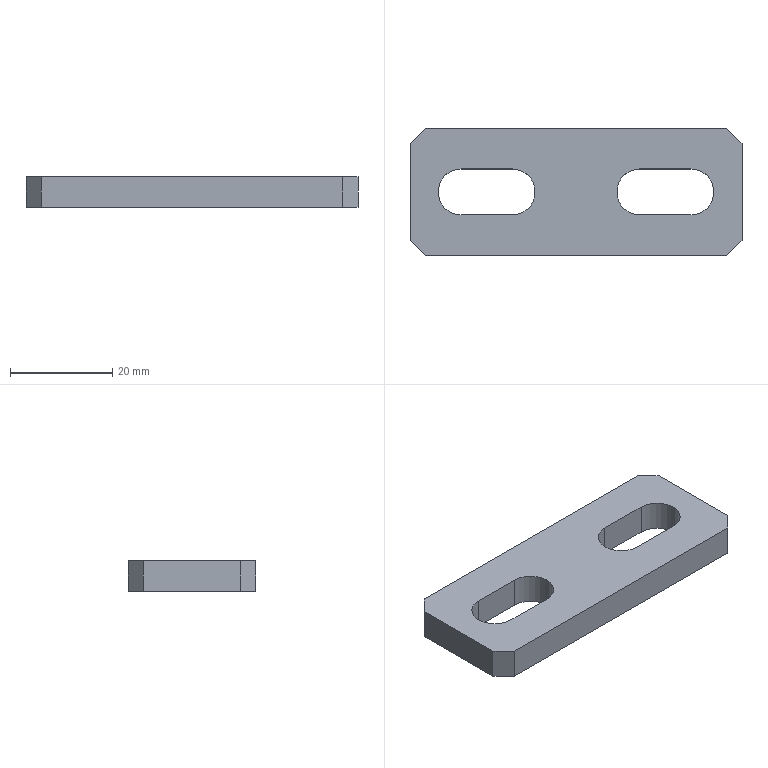Part | STEP file | linkfor guide | 1 solid | 18 faces | box 65 x 25 x 6 mm | volume 7799 mm3 | plane 14 | cylinder 4 | commonest cylinder face diameters 9 x4
STEP:
#1=CARTESIAN_POINT('',(0.,0.,0.));
#2=DIRECTION('',(0.,0.,1.));
#3=DIRECTION('',(1.,0.,0.));
#4=AXIS2_PLACEMENT_3D('',#1,#2,#3);
#5=CARTESIAN_POINT('',(45.,-10.346,6.));
#6=VERTEX_POINT('',#5);
#7=CARTESIAN_POINT('',(45.,-10.346,0.));
#8=VERTEX_POINT('',#7);
#9=CARTESIAN_POINT('',(45.,-10.346,6.));
#10=DIRECTION('',(0.,0.,-1.));
#11=VECTOR('',#10,1.);
#12=LINE('',#9,#11);
#13=CARTESIAN_POINT('',(45.,-5.846,6.));
#14=DIRECTION('',(0.,0.,-1.));
#15=DIRECTION('',(0.,1.,0.));
#16=AXIS2_PLACEMENT_3D('',#13,#14,#15);
#17=CYLINDRICAL_SURFACE('',#16,4.5);
#18=CARTESIAN_POINT('',(3.142,0.));
#19=DIRECTION('',(0.,1.));
#20=VECTOR('',#19,1.);
#21=LINE('',#18,#20);
#22=(GEOMETRIC_REPRESENTATION_CONTEXT(2)PARAMETRIC_REPRESENTATION_CONTEXT()REPRESENTATION_CONTEXT('',''));
#23=DEFINITIONAL_REPRESENTATION('',(#21),#22);
#24=PCURVE('',#17,#23);
#25=CARTESIAN_POINT('',(45.,-10.346,6.));
#26=DIRECTION('',(0.,-1.,0.));
#27=DIRECTION('',(0.,0.,-1.));
#28=AXIS2_PLACEMENT_3D('',#25,#26,#27);
#29=PLANE('',#28);
#30=CARTESIAN_POINT('',(0.,0.));
#31=DIRECTION('',(1.,0.));
#32=VECTOR('',#31,1.);
#33=LINE('',#30,#32);
#34=(GEOMETRIC_REPRESENTATION_CONTEXT(2)PARAMETRIC_REPRESENTATION_CONTEXT()REPRESENTATION_CONTEXT('',''));
#35=DEFINITIONAL_REPRESENTATION('',(#33),#34);
#36=PCURVE('',#29,#35);
#37=SURFACE_CURVE('',#12,(#24,#36),.PCURVE_S1.);
#38=EDGE_CURVE('',#6,#8,#37,.T.);
#39=ORIENTED_EDGE('',*,*,#38,.F.);
#40=CARTESIAN_POINT('',(45.,-1.346,6.));
#41=VERTEX_POINT('',#40);
#42=CARTESIAN_POINT('',(45.,-5.846,6.));
#43=DIRECTION('',(0.,0.,-1.));
#44=DIRECTION('',(0.,1.,0.));
#45=AXIS2_PLACEMENT_3D('',#42,#43,#44);
#46=CIRCLE('',#45,4.5);
#47=CARTESIAN_POINT('',(0.,0.));
#48=DIRECTION('',(1.,0.));
#49=VECTOR('',#48,1.);
#50=LINE('',#47,#49);
#51=(GEOMETRIC_REPRESENTATION_CONTEXT(2)PARAMETRIC_REPRESENTATION_CONTEXT()REPRESENTATION_CONTEXT('',''));
#52=DEFINITIONAL_REPRESENTATION('',(#50),#51);
#53=PCURVE('',#17,#52);
#54=CARTESIAN_POINT('',(32.5,-5.846,6.));
#55=DIRECTION('',(0.,0.,1.));
#56=DIRECTION('',(1.,0.,0.));
#57=AXIS2_PLACEMENT_3D('',#54,#55,#56);
#58=PLANE('',#57);
#59=CARTESIAN_POINT('',(12.5,4.5));
#60=CARTESIAN_POINT('',(20.294,4.5));
#61=CARTESIAN_POINT('',(16.397,-2.25));
#62=CARTESIAN_POINT('',(12.5,-9.));
#63=CARTESIAN_POINT('',(8.603,-2.25));
#64=CARTESIAN_POINT('',(4.706,4.5));
#65=CARTESIAN_POINT('',(12.5,4.5));
#66=(BOUNDED_CURVE()B_SPLINE_CURVE(2,(#59,#60,#61,#62,#63,#64,#65),.UNSPECIFIED.,.T.,.F.)B_SPLINE_CURVE_WITH_KNOTS((1,2,2,2,2,1),(-2.094,0.,2.094,4.189,6.283,8.378),.UNSPECIFIED.)CURVE()GEOMETRIC_REPRESENTATION_ITEM()RATIONAL_B_SPLINE_CURVE((1.,0.5,1.,0.5,1.,0.5,1.))REPRESENTATION_ITEM(''));
#67=(GEOMETRIC_REPRESENTATION_CONTEXT(2)PARAMETRIC_REPRESENTATION_CONTEXT()REPRESENTATION_CONTEXT('',''));
#68=DEFINITIONAL_REPRESENTATION('',(#66),#67);
#69=PCURVE('',#58,#68);
#70=SURFACE_CURVE('',#46,(#53,#69),.PCURVE_S1.);
#71=EDGE_CURVE('',#6,#41,#70,.T.);
#72=ORIENTED_EDGE('',*,*,#71,.T.);
#73=CARTESIAN_POINT('',(45.,-1.346,0.));
#74=VERTEX_POINT('',#73);
#75=CARTESIAN_POINT('',(45.,-1.346,6.));
#76=DIRECTION('',(0.,0.,-1.));
#77=VECTOR('',#76,1.);
#78=LINE('',#75,#77);
#79=CARTESIAN_POINT('',(6.283,0.));
#80=DIRECTION('',(0.,1.));
#81=VECTOR('',#80,1.);
#82=LINE('',#79,#81);
#83=(GEOMETRIC_REPRESENTATION_CONTEXT(2)PARAMETRIC_REPRESENTATION_CONTEXT()REPRESENTATION_CONTEXT('',''));
#84=DEFINITIONAL_REPRESENTATION('',(#82),#83);
#85=PCURVE('',#17,#84);
#86=CARTESIAN_POINT('',(55.,-1.346,6.));
#87=DIRECTION('',(0.,1.,0.));
#88=DIRECTION('',(0.,0.,1.));
#89=AXIS2_PLACEMENT_3D('',#86,#87,#88);
#90=PLANE('',#89);
#91=CARTESIAN_POINT('',(0.,-10.));
#92=DIRECTION('',(-1.,0.));
#93=VECTOR('',#92,1.);
#94=LINE('',#91,#93);
#95=(GEOMETRIC_REPRESENTATION_CONTEXT(2)PARAMETRIC_REPRESENTATION_CONTEXT()REPRESENTATION_CONTEXT('',''));
#96=DEFINITIONAL_REPRESENTATION('',(#94),#95);
#97=PCURVE('',#90,#96);
#98=SURFACE_CURVE('',#78,(#85,#97),.PCURVE_S1.);
#99=EDGE_CURVE('',#41,#74,#98,.T.);
#100=ORIENTED_EDGE('',*,*,#99,.T.);
#101=CARTESIAN_POINT('',(45.,-5.846,0.));
#102=DIRECTION('',(0.,0.,1.));
#103=DIRECTION('',(0.,1.,0.));
#104=AXIS2_PLACEMENT_3D('',#101,#102,#103);
#105=CIRCLE('',#104,4.5);
#106=CARTESIAN_POINT('',(6.283,6.));
#107=DIRECTION('',(-1.,0.));
#108=VECTOR('',#107,1.);
#109=LINE('',#106,#108);
#110=(GEOMETRIC_REPRESENTATION_CONTEXT(2)PARAMETRIC_REPRESENTATION_CONTEXT()REPRESENTATION_CONTEXT('',''));
#111=DEFINITIONAL_REPRESENTATION('',(#109),#110);
#112=PCURVE('',#17,#111);
#113=CARTESIAN_POINT('',(32.5,-5.846,0.));
#114=DIRECTION('',(0.,0.,1.));
#115=DIRECTION('',(1.,0.,0.));
#116=AXIS2_PLACEMENT_3D('',#113,#114,#115);
#117=PLANE('',#116);
#118=CARTESIAN_POINT('',(12.5,0.));
#119=DIRECTION('',(0.,1.));
#120=AXIS2_PLACEMENT_2D('',#118,#119);
#121=CIRCLE('',#120,4.5);
#122=(GEOMETRIC_REPRESENTATION_CONTEXT(2)PARAMETRIC_REPRESENTATION_CONTEXT()REPRESENTATION_CONTEXT('',''));
#123=DEFINITIONAL_REPRESENTATION('',(#121),#122);
#124=PCURVE('',#117,#123);
#125=SURFACE_CURVE('',#105,(#112,#124),.PCURVE_S1.);
#126=EDGE_CURVE('',#74,#8,#125,.T.);
#127=ORIENTED_EDGE('',*,*,#126,.T.);
#128=EDGE_LOOP('',(#39,#72,#100,#127));
#129=FACE_BOUND('',#128,.F.);
#130=ADVANCED_FACE('',(#129),#17,.F.);
#131=CARTESIAN_POINT('',(55.,-10.346,0.));
#132=VERTEX_POINT('',#131);
#133=CARTESIAN_POINT('',(45.,-10.346,0.));
#134=DIRECTION('',(1.,0.,0.));
#135=VECTOR('',#134,1.);
#136=LINE('',#133,#135);
#137=CARTESIAN_POINT('',(6.,0.));
#138=DIRECTION('',(0.,1.));
#139=VECTOR('',#138,1.);
#140=LINE('',#137,#139);
#141=(GEOMETRIC_REPRESENTATION_CONTEXT(2)PARAMETRIC_REPRESENTATION_CONTEXT()REPRESENTATION_CONTEXT('',''));
#142=DEFINITIONAL_REPRESENTATION('',(#140),#141);
#143=PCURVE('',#29,#142);
#144=CARTESIAN_POINT('',(12.5,-4.5));
#145=DIRECTION('',(1.,0.));
#146=VECTOR('',#145,1.);
#147=LINE('',#144,#146);
#148=(GEOMETRIC_REPRESENTATION_CONTEXT(2)PARAMETRIC_REPRESENTATION_CONTEXT()REPRESENTATION_CONTEXT('',''));
#149=DEFINITIONAL_REPRESENTATION('',(#147),#148);
#150=PCURVE('',#117,#149);
#151=SURFACE_CURVE('',#136,(#143,#150),.PCURVE_S1.);
#152=EDGE_CURVE('',#8,#132,#151,.T.);
#153=ORIENTED_EDGE('',*,*,#152,.F.);
#154=ORIENTED_EDGE('',*,*,#38,.F.);
#155=CARTESIAN_POINT('',(55.,-10.346,6.));
#156=VERTEX_POINT('',#155);
#157=CARTESIAN_POINT('',(55.,-10.346,6.));
#158=DIRECTION('',(-1.,0.,0.));
#159=VECTOR('',#158,1.);
#160=LINE('',#157,#159);
#161=CARTESIAN_POINT('',(0.,10.));
#162=DIRECTION('',(0.,-1.));
#163=VECTOR('',#162,1.);
#164=LINE('',#161,#163);
#165=(GEOMETRIC_REPRESENTATION_CONTEXT(2)PARAMETRIC_REPRESENTATION_CONTEXT()REPRESENTATION_CONTEXT('',''));
#166=DEFINITIONAL_REPRESENTATION('',(#164),#165);
#167=PCURVE('',#29,#166);
#168=CARTESIAN_POINT('',(22.5,-4.5));
#169=DIRECTION('',(-1.,0.));
#170=VECTOR('',#169,1.);
#171=LINE('',#168,#170);
#172=(GEOMETRIC_REPRESENTATION_CONTEXT(2)PARAMETRIC_REPRESENTATION_CONTEXT()REPRESENTATION_CONTEXT('',''));
#173=DEFINITIONAL_REPRESENTATION('',(#171),#172);
#174=PCURVE('',#58,#173);
#175=SURFACE_CURVE('',#160,(#167,#174),.PCURVE_S1.);
#176=EDGE_CURVE('',#156,#6,#175,.T.);
#177=ORIENTED_EDGE('',*,*,#176,.F.);
#178=CARTESIAN_POINT('',(55.,-10.346,6.));
#179=DIRECTION('',(0.,0.,-1.));
#180=VECTOR('',#179,1.);
#181=LINE('',#178,#180);
#182=CARTESIAN_POINT('',(0.,10.));
#183=DIRECTION('',(1.,0.));
#184=VECTOR('',#183,1.);
#185=LINE('',#182,#184);
#186=(GEOMETRIC_REPRESENTATION_CONTEXT(2)PARAMETRIC_REPRESENTATION_CONTEXT()REPRESENTATION_CONTEXT('',''));
#187=DEFINITIONAL_REPRESENTATION('',(#185),#186);
#188=PCURVE('',#29,#187);
#189=CARTESIAN_POINT('',(55.,-5.846,6.));
#190=DIRECTION('',(0.,0.,-1.));
#191=DIRECTION('',(0.,-1.,0.));
#192=AXIS2_PLACEMENT_3D('',#189,#190,#191);
#193=CYLINDRICAL_SURFACE('',#192,4.5);
#194=CARTESIAN_POINT('',(6.283,0.));
#195=DIRECTION('',(0.,1.));
#196=VECTOR('',#195,1.);
#197=LINE('',#194,#196);
#198=(GEOMETRIC_REPRESENTATION_CONTEXT(2)PARAMETRIC_REPRESENTATION_CONTEXT()REPRESENTATION_CONTEXT('',''));
#199=DEFINITIONAL_REPRESENTATION('',(#197),#198);
#200=PCURVE('',#193,#199);
#201=SURFACE_CURVE('',#181,(#188,#200),.PCURVE_S1.);
#202=EDGE_CURVE('',#156,#132,#201,.T.);
#203=ORIENTED_EDGE('',*,*,#202,.T.);
#204=EDGE_LOOP('',(#153,#154,#177,#203));
#205=FACE_BOUND('',#204,.T.);
#206=ADVANCED_FACE('',(#205),#29,.F.);
#207=CARTESIAN_POINT('',(55.,-1.346,6.));
#208=VERTEX_POINT('',#207);
#209=CARTESIAN_POINT('',(55.,-1.346,0.));
#210=VERTEX_POINT('',#209);
#211=CARTESIAN_POINT('',(55.,-1.346,6.));
#212=DIRECTION('',(0.,0.,-1.));
#213=VECTOR('',#212,1.);
#214=LINE('',#211,#213);
#215=CARTESIAN_POINT('',(3.142,0.));
#216=DIRECTION('',(0.,1.));
#217=VECTOR('',#216,1.);
#218=LINE('',#215,#217);
#219=(GEOMETRIC_REPRESENTATION_CONTEXT(2)PARAMETRIC_REPRESENTATION_CONTEXT()REPRESENTATION_CONTEXT('',''));
#220=DEFINITIONAL_REPRESENTATION('',(#218),#219);
#221=PCURVE('',#193,#220);
#222=CARTESIAN_POINT('',(0.,0.));
#223=DIRECTION('',(-1.,0.));
#224=VECTOR('',#223,1.);
#225=LINE('',#222,#224);
#226=(GEOMETRIC_REPRESENTATION_CONTEXT(2)PARAMETRIC_REPRESENTATION_CONTEXT()REPRESENTATION_CONTEXT('',''));
#227=DEFINITIONAL_REPRESENTATION('',(#225),#226);
#228=PCURVE('',#90,#227);
#229=SURFACE_CURVE('',#214,(#221,#228),.PCURVE_S1.);
#230=EDGE_CURVE('',#208,#210,#229,.T.);
#231=ORIENTED_EDGE('',*,*,#230,.F.);
#232=CARTESIAN_POINT('',(55.,-5.846,6.));
#233=DIRECTION('',(0.,0.,-1.));
#234=DIRECTION('',(0.,-1.,0.));
#235=AXIS2_PLACEMENT_3D('',#232,#233,#234);
#236=CIRCLE('',#235,4.5);
#237=CARTESIAN_POINT('',(0.,0.));
#238=DIRECTION('',(1.,0.));
#239=VECTOR('',#238,1.);
#240=LINE('',#237,#239);
#241=(GEOMETRIC_REPRESENTATION_CONTEXT(2)PARAMETRIC_REPRESENTATION_CONTEXT()REPRESENTATION_CONTEXT('',''));
#242=DEFINITIONAL_REPRESENTATION('',(#240),#241);
#243=PCURVE('',#193,#242);
#244=CARTESIAN_POINT('',(22.5,-4.5));
#245=CARTESIAN_POINT('',(14.706,-4.5));
#246=CARTESIAN_POINT('',(18.603,2.25));
#247=CARTESIAN_POINT('',(22.5,9.));
#248=CARTESIAN_POINT('',(26.397,2.25));
#249=CARTESIAN_POINT('',(30.294,-4.5));
#250=CARTESIAN_POINT('',(22.5,-4.5));
#251=(BOUNDED_CURVE()B_SPLINE_CURVE(2,(#244,#245,#246,#247,#248,#249,#250),.UNSPECIFIED.,.T.,.F.)B_SPLINE_CURVE_WITH_KNOTS((1,2,2,2,2,1),(-2.094,0.,2.094,4.189,6.283,8.378),.UNSPECIFIED.)CURVE()GEOMETRIC_REPRESENTATION_ITEM()RATIONAL_B_SPLINE_CURVE((1.,0.5,1.,0.5,1.,0.5,1.))REPRESENTATION_ITEM(''));
#252=(GEOMETRIC_REPRESENTATION_CONTEXT(2)PARAMETRIC_REPRESENTATION_CONTEXT()REPRESENTATION_CONTEXT('',''));
#253=DEFINITIONAL_REPRESENTATION('',(#251),#252);
#254=PCURVE('',#58,#253);
#255=SURFACE_CURVE('',#236,(#243,#254),.PCURVE_S1.);
#256=EDGE_CURVE('',#208,#156,#255,.T.);
#257=ORIENTED_EDGE('',*,*,#256,.T.);
#258=ORIENTED_EDGE('',*,*,#202,.T.);
#259=CARTESIAN_POINT('',(55.,-5.846,0.));
#260=DIRECTION('',(0.,0.,1.));
#261=DIRECTION('',(0.,-1.,0.));
#262=AXIS2_PLACEMENT_3D('',#259,#260,#261);
#263=CIRCLE('',#262,4.5);
#264=CARTESIAN_POINT('',(6.283,6.));
#265=DIRECTION('',(-1.,0.));
#266=VECTOR('',#265,1.);
#267=LINE('',#264,#266);
#268=(GEOMETRIC_REPRESENTATION_CONTEXT(2)PARAMETRIC_REPRESENTATION_CONTEXT()REPRESENTATION_CONTEXT('',''));
#269=DEFINITIONAL_REPRESENTATION('',(#267),#268);
#270=PCURVE('',#193,#269);
#271=CARTESIAN_POINT('',(22.5,0.));
#272=DIRECTION('',(0.,-1.));
#273=AXIS2_PLACEMENT_2D('',#271,#272);
#274=CIRCLE('',#273,4.5);
#275=(GEOMETRIC_REPRESENTATION_CONTEXT(2)PARAMETRIC_REPRESENTATION_CONTEXT()REPRESENTATION_CONTEXT('',''));
#276=DEFINITIONAL_REPRESENTATION('',(#274),#275);
#277=PCURVE('',#117,#276);
#278=SURFACE_CURVE('',#263,(#270,#277),.PCURVE_S1.);
#279=EDGE_CURVE('',#132,#210,#278,.T.);
#280=ORIENTED_EDGE('',*,*,#279,.T.);
#281=EDGE_LOOP('',(#231,#257,#258,#280));
#282=FACE_BOUND('',#281,.F.);
#283=ADVANCED_FACE('',(#282),#193,.F.);
#284=CARTESIAN_POINT('',(55.,-1.346,0.));
#285=DIRECTION('',(-1.,0.,0.));
#286=VECTOR('',#285,1.);
#287=LINE('',#284,#286);
#288=CARTESIAN_POINT('',(-6.,0.));
#289=DIRECTION('',(0.,-1.));
#290=VECTOR('',#289,1.);
#291=LINE('',#288,#290);
#292=(GEOMETRIC_REPRESENTATION_CONTEXT(2)PARAMETRIC_REPRESENTATION_CONTEXT()REPRESENTATION_CONTEXT('',''));
#293=DEFINITIONAL_REPRESENTATION('',(#291),#292);
#294=PCURVE('',#90,#293);
#295=CARTESIAN_POINT('',(22.5,4.5));
#296=DIRECTION('',(-1.,0.));
#297=VECTOR('',#296,1.);
#298=LINE('',#295,#297);
#299=(GEOMETRIC_REPRESENTATION_CONTEXT(2)PARAMETRIC_REPRESENTATION_CONTEXT()REPRESENTATION_CONTEXT('',''));
#300=DEFINITIONAL_REPRESENTATION('',(#298),#299);
#301=PCURVE('',#117,#300);
#302=SURFACE_CURVE('',#287,(#294,#301),.PCURVE_S1.);
#303=EDGE_CURVE('',#210,#74,#302,.T.);
#304=ORIENTED_EDGE('',*,*,#303,.F.);
#305=ORIENTED_EDGE('',*,*,#230,.F.);
#306=CARTESIAN_POINT('',(45.,-1.346,6.));
#307=DIRECTION('',(1.,0.,0.));
#308=VECTOR('',#307,1.);
#309=LINE('',#306,#308);
#310=CARTESIAN_POINT('',(0.,-10.));
#311=DIRECTION('',(0.,1.));
#312=VECTOR('',#311,1.);
#313=LINE('',#310,#312);
#314=(GEOMETRIC_REPRESENTATION_CONTEXT(2)PARAMETRIC_REPRESENTATION_CONTEXT()REPRESENTATION_CONTEXT('',''));
#315=DEFINITIONAL_REPRESENTATION('',(#313),#314);
#316=PCURVE('',#90,#315);
#317=CARTESIAN_POINT('',(12.5,4.5));
#318=DIRECTION('',(1.,0.));
#319=VECTOR('',#318,1.);
#320=LINE('',#317,#319);
#321=(GEOMETRIC_REPRESENTATION_CONTEXT(2)PARAMETRIC_REPRESENTATION_CONTEXT()REPRESENTATION_CONTEXT('',''));
#322=DEFINITIONAL_REPRESENTATION('',(#320),#321);
#323=PCURVE('',#58,#322);
#324=SURFACE_CURVE('',#309,(#316,#323),.PCURVE_S1.);
#325=EDGE_CURVE('',#41,#208,#324,.T.);
#326=ORIENTED_EDGE('',*,*,#325,.F.);
#327=ORIENTED_EDGE('',*,*,#99,.T.);
#328=EDGE_LOOP('',(#304,#305,#326,#327));
#329=FACE_BOUND('',#328,.T.);
#330=ADVANCED_FACE('',(#329),#90,.F.);
#331=CARTESIAN_POINT('',(20.,-1.346,6.));
#332=VERTEX_POINT('',#331);
#333=CARTESIAN_POINT('',(20.,-1.346,0.));
#334=VERTEX_POINT('',#333);
#335=CARTESIAN_POINT('',(20.,-1.346,6.));
#336=DIRECTION('',(0.,0.,-1.));
#337=VECTOR('',#336,1.);
#338=LINE('',#335,#337);
#339=CARTESIAN_POINT('',(20.,-5.846,6.));
#340=DIRECTION('',(0.,0.,-1.));
#341=DIRECTION('',(0.,1.,0.));
#342=AXIS2_PLACEMENT_3D('',#339,#340,#341);
#343=CYLINDRICAL_SURFACE('',#342,4.5);
#344=CARTESIAN_POINT('',(0.,0.));
#345=DIRECTION('',(0.,1.));
#346=VECTOR('',#345,1.);
#347=LINE('',#344,#346);
#348=(GEOMETRIC_REPRESENTATION_CONTEXT(2)PARAMETRIC_REPRESENTATION_CONTEXT()REPRESENTATION_CONTEXT('',''));
#349=DEFINITIONAL_REPRESENTATION('',(#347),#348);
#350=PCURVE('',#343,#349);
#351=CARTESIAN_POINT('',(20.,-1.346,6.));
#352=DIRECTION('',(0.,1.,0.));
#353=DIRECTION('',(0.,0.,1.));
#354=AXIS2_PLACEMENT_3D('',#351,#352,#353);
#355=PLANE('',#354);
#356=CARTESIAN_POINT('',(0.,0.));
#357=DIRECTION('',(-1.,0.));
#358=VECTOR('',#357,1.);
#359=LINE('',#356,#358);
#360=(GEOMETRIC_REPRESENTATION_CONTEXT(2)PARAMETRIC_REPRESENTATION_CONTEXT()REPRESENTATION_CONTEXT('',''));
#361=DEFINITIONAL_REPRESENTATION('',(#359),#360);
#362=PCURVE('',#355,#361);
#363=SURFACE_CURVE('',#338,(#350,#362),.PCURVE_S1.);
#364=EDGE_CURVE('',#332,#334,#363,.T.);
#365=ORIENTED_EDGE('',*,*,#364,.F.);
#366=CARTESIAN_POINT('',(20.,-10.346,6.));
#367=VERTEX_POINT('',#366);
#368=CARTESIAN_POINT('',(20.,-5.846,6.));
#369=DIRECTION('',(0.,0.,-1.));
#370=DIRECTION('',(0.,1.,0.));
#371=AXIS2_PLACEMENT_3D('',#368,#369,#370);
#372=CIRCLE('',#371,4.5);
#373=CARTESIAN_POINT('',(0.,0.));
#374=DIRECTION('',(1.,0.));
#375=VECTOR('',#374,1.);
#376=LINE('',#373,#375);
#377=(GEOMETRIC_REPRESENTATION_CONTEXT(2)PARAMETRIC_REPRESENTATION_CONTEXT()REPRESENTATION_CONTEXT('',''));
#378=DEFINITIONAL_REPRESENTATION('',(#376),#377);
#379=PCURVE('',#343,#378);
#380=CARTESIAN_POINT('',(-12.5,4.5));
#381=CARTESIAN_POINT('',(-4.706,4.5));
#382=CARTESIAN_POINT('',(-8.603,-2.25));
#383=CARTESIAN_POINT('',(-12.5,-9.));
#384=CARTESIAN_POINT('',(-16.397,-2.25));
#385=CARTESIAN_POINT('',(-20.294,4.5));
#386=CARTESIAN_POINT('',(-12.5,4.5));
#387=(BOUNDED_CURVE()B_SPLINE_CURVE(2,(#380,#381,#382,#383,#384,#385,#386),.UNSPECIFIED.,.T.,.F.)B_SPLINE_CURVE_WITH_KNOTS((1,2,2,2,2,1),(-2.094,0.,2.094,4.189,6.283,8.378),.UNSPECIFIED.)CURVE()GEOMETRIC_REPRESENTATION_ITEM()RATIONAL_B_SPLINE_CURVE((1.,0.5,1.,0.5,1.,0.5,1.))REPRESENTATION_ITEM(''));
#388=(GEOMETRIC_REPRESENTATION_CONTEXT(2)PARAMETRIC_REPRESENTATION_CONTEXT()REPRESENTATION_CONTEXT('',''));
#389=DEFINITIONAL_REPRESENTATION('',(#387),#388);
#390=PCURVE('',#58,#389);
#391=SURFACE_CURVE('',#372,(#379,#390),.PCURVE_S1.);
#392=EDGE_CURVE('',#332,#367,#391,.T.);
#393=ORIENTED_EDGE('',*,*,#392,.T.);
#394=CARTESIAN_POINT('',(20.,-10.346,0.));
#395=VERTEX_POINT('',#394);
#396=CARTESIAN_POINT('',(20.,-10.346,6.));
#397=DIRECTION('',(0.,0.,-1.));
#398=VECTOR('',#397,1.);
#399=LINE('',#396,#398);
#400=CARTESIAN_POINT('',(3.142,0.));
#401=DIRECTION('',(0.,1.));
#402=VECTOR('',#401,1.);
#403=LINE('',#400,#402);
#404=(GEOMETRIC_REPRESENTATION_CONTEXT(2)PARAMETRIC_REPRESENTATION_CONTEXT()REPRESENTATION_CONTEXT('',''));
#405=DEFINITIONAL_REPRESENTATION('',(#403),#404);
#406=PCURVE('',#343,#405);
#407=CARTESIAN_POINT('',(10.,-10.346,6.));
#408=DIRECTION('',(0.,-1.,0.));
#409=DIRECTION('',(0.,0.,-1.));
#410=AXIS2_PLACEMENT_3D('',#407,#408,#409);
#411=PLANE('',#410);
#412=CARTESIAN_POINT('',(0.,10.));
#413=DIRECTION('',(1.,0.));
#414=VECTOR('',#413,1.);
#415=LINE('',#412,#414);
#416=(GEOMETRIC_REPRESENTATION_CONTEXT(2)PARAMETRIC_REPRESENTATION_CONTEXT()REPRESENTATION_CONTEXT('',''));
#417=DEFINITIONAL_REPRESENTATION('',(#415),#416);
#418=PCURVE('',#411,#417);
#419=SURFACE_CURVE('',#399,(#406,#418),.PCURVE_S1.);
#420=EDGE_CURVE('',#367,#395,#419,.T.);
#421=ORIENTED_EDGE('',*,*,#420,.T.);
#422=CARTESIAN_POINT('',(20.,-5.846,0.));
#423=DIRECTION('',(0.,0.,1.));
#424=DIRECTION('',(0.,1.,0.));
#425=AXIS2_PLACEMENT_3D('',#422,#423,#424);
#426=CIRCLE('',#425,4.5);
#427=CARTESIAN_POINT('',(6.283,6.));
#428=DIRECTION('',(-1.,0.));
#429=VECTOR('',#428,1.);
#430=LINE('',#427,#429);
#431=(GEOMETRIC_REPRESENTATION_CONTEXT(2)PARAMETRIC_REPRESENTATION_CONTEXT()REPRESENTATION_CONTEXT('',''));
#432=DEFINITIONAL_REPRESENTATION('',(#430),#431);
#433=PCURVE('',#343,#432);
#434=CARTESIAN_POINT('',(-12.5,0.));
#435=DIRECTION('',(0.,1.));
#436=AXIS2_PLACEMENT_2D('',#434,#435);
#437=CIRCLE('',#436,4.5);
#438=(GEOMETRIC_REPRESENTATION_CONTEXT(2)PARAMETRIC_REPRESENTATION_CONTEXT()REPRESENTATION_CONTEXT('',''));
#439=DEFINITIONAL_REPRESENTATION('',(#437),#438);
#440=PCURVE('',#117,#439);
#441=SURFACE_CURVE('',#426,(#433,#440),.PCURVE_S1.);
#442=EDGE_CURVE('',#395,#334,#441,.T.);
#443=ORIENTED_EDGE('',*,*,#442,.T.);
#444=EDGE_LOOP('',(#365,#393,#421,#443));
#445=FACE_BOUND('',#444,.F.);
#446=ADVANCED_FACE('',(#445),#343,.F.);
#447=CARTESIAN_POINT('',(10.,-1.346,0.));
#448=VERTEX_POINT('',#447);
#449=CARTESIAN_POINT('',(20.,-1.346,0.));
#450=DIRECTION('',(-1.,0.,0.));
#451=VECTOR('',#450,1.);
#452=LINE('',#449,#451);
#453=CARTESIAN_POINT('',(-6.,0.));
#454=DIRECTION('',(0.,-1.));
#455=VECTOR('',#454,1.);
#456=LINE('',#453,#455);
#457=(GEOMETRIC_REPRESENTATION_CONTEXT(2)PARAMETRIC_REPRESENTATION_CONTEXT()REPRESENTATION_CONTEXT('',''));
#458=DEFINITIONAL_REPRESENTATION('',(#456),#457);
#459=PCURVE('',#355,#458);
#460=CARTESIAN_POINT('',(-12.5,4.5));
#461=DIRECTION('',(-1.,0.));
#462=VECTOR('',#461,1.);
#463=LINE('',#460,#462);
#464=(GEOMETRIC_REPRESENTATION_CONTEXT(2)PARAMETRIC_REPRESENTATION_CONTEXT()REPRESENTATION_CONTEXT('',''));
#465=DEFINITIONAL_REPRESENTATION('',(#463),#464);
#466=PCURVE('',#117,#465);
#467=SURFACE_CURVE('',#452,(#459,#466),.PCURVE_S1.);
#468=EDGE_CURVE('',#334,#448,#467,.T.);
#469=ORIENTED_EDGE('',*,*,#468,.F.);
#470=ORIENTED_EDGE('',*,*,#364,.F.);
#471=CARTESIAN_POINT('',(10.,-1.346,6.));
#472=VERTEX_POINT('',#471);
#473=CARTESIAN_POINT('',(10.,-1.346,6.));
#474=DIRECTION('',(1.,0.,0.));
#475=VECTOR('',#474,1.);
#476=LINE('',#473,#475);
#477=CARTESIAN_POINT('',(0.,-10.));
#478=DIRECTION('',(0.,1.));
#479=VECTOR('',#478,1.);
#480=LINE('',#477,#479);
#481=(GEOMETRIC_REPRESENTATION_CONTEXT(2)PARAMETRIC_REPRESENTATION_CONTEXT()REPRESENTATION_CONTEXT('',''));
#482=DEFINITIONAL_REPRESENTATION('',(#480),#481);
#483=PCURVE('',#355,#482);
#484=CARTESIAN_POINT('',(-22.5,4.5));
#485=DIRECTION('',(1.,0.));
#486=VECTOR('',#485,1.);
#487=LINE('',#484,#486);
#488=(GEOMETRIC_REPRESENTATION_CONTEXT(2)PARAMETRIC_REPRESENTATION_CONTEXT()REPRESENTATION_CONTEXT('',''));
#489=DEFINITIONAL_REPRESENTATION('',(#487),#488);
#490=PCURVE('',#58,#489);
#491=SURFACE_CURVE('',#476,(#483,#490),.PCURVE_S1.);
#492=EDGE_CURVE('',#472,#332,#491,.T.);
#493=ORIENTED_EDGE('',*,*,#492,.F.);
#494=CARTESIAN_POINT('',(10.,-1.346,6.));
#495=DIRECTION('',(0.,0.,-1.));
#496=VECTOR('',#495,1.);
#497=LINE('',#494,#496);
#498=CARTESIAN_POINT('',(0.,-10.));
#499=DIRECTION('',(-1.,0.));
#500=VECTOR('',#499,1.);
#501=LINE('',#498,#500);
#502=(GEOMETRIC_REPRESENTATION_CONTEXT(2)PARAMETRIC_REPRESENTATION_CONTEXT()REPRESENTATION_CONTEXT('',''));
#503=DEFINITIONAL_REPRESENTATION('',(#501),#502);
#504=PCURVE('',#355,#503);
#505=CARTESIAN_POINT('',(10.,-5.846,6.));
#506=DIRECTION('',(0.,0.,-1.));
#507=DIRECTION('',(0.,-1.,0.));
#508=AXIS2_PLACEMENT_3D('',#505,#506,#507);
#509=CYLINDRICAL_SURFACE('',#508,4.5);
#510=CARTESIAN_POINT('',(3.142,0.));
#511=DIRECTION('',(0.,1.));
#512=VECTOR('',#511,1.);
#513=LINE('',#510,#512);
#514=(GEOMETRIC_REPRESENTATION_CONTEXT(2)PARAMETRIC_REPRESENTATION_CONTEXT()REPRESENTATION_CONTEXT('',''));
#515=DEFINITIONAL_REPRESENTATION('',(#513),#514);
#516=PCURVE('',#509,#515);
#517=SURFACE_CURVE('',#497,(#504,#516),.PCURVE_S1.);
#518=EDGE_CURVE('',#472,#448,#517,.T.);
#519=ORIENTED_EDGE('',*,*,#518,.T.);
#520=EDGE_LOOP('',(#469,#470,#493,#519));
#521=FACE_BOUND('',#520,.T.);
#522=ADVANCED_FACE('',(#521),#355,.F.);
#523=CARTESIAN_POINT('',(10.,-10.346,6.));
#524=VERTEX_POINT('',#523);
#525=CARTESIAN_POINT('',(10.,-10.346,0.));
#526=VERTEX_POINT('',#525);
#527=CARTESIAN_POINT('',(10.,-10.346,6.));
#528=DIRECTION('',(0.,0.,-1.));
#529=VECTOR('',#528,1.);
#530=LINE('',#527,#529);
#531=CARTESIAN_POINT('',(0.,0.));
#532=DIRECTION('',(0.,1.));
#533=VECTOR('',#532,1.);
#534=LINE('',#531,#533);
#535=(GEOMETRIC_REPRESENTATION_CONTEXT(2)PARAMETRIC_REPRESENTATION_CONTEXT()REPRESENTATION_CONTEXT('',''));
#536=DEFINITIONAL_REPRESENTATION('',(#534),#535);
#537=PCURVE('',#509,#536);
#538=CARTESIAN_POINT('',(0.,0.));
#539=DIRECTION('',(1.,0.));
#540=VECTOR('',#539,1.);
#541=LINE('',#538,#540);
#542=(GEOMETRIC_REPRESENTATION_CONTEXT(2)PARAMETRIC_REPRESENTATION_CONTEXT()REPRESENTATION_CONTEXT('',''));
#543=DEFINITIONAL_REPRESENTATION('',(#541),#542);
#544=PCURVE('',#411,#543);
#545=SURFACE_CURVE('',#530,(#537,#544),.PCURVE_S1.);
#546=EDGE_CURVE('',#524,#526,#545,.T.);
#547=ORIENTED_EDGE('',*,*,#546,.F.);
#548=CARTESIAN_POINT('',(10.,-5.846,6.));
#549=DIRECTION('',(0.,0.,-1.));
#550=DIRECTION('',(0.,-1.,0.));
#551=AXIS2_PLACEMENT_3D('',#548,#549,#550);
#552=CIRCLE('',#551,4.5);
#553=CARTESIAN_POINT('',(0.,0.));
#554=DIRECTION('',(1.,0.));
#555=VECTOR('',#554,1.);
#556=LINE('',#553,#555);
#557=(GEOMETRIC_REPRESENTATION_CONTEXT(2)PARAMETRIC_REPRESENTATION_CONTEXT()REPRESENTATION_CONTEXT('',''));
#558=DEFINITIONAL_REPRESENTATION('',(#556),#557);
#559=PCURVE('',#509,#558);
#560=CARTESIAN_POINT('',(-22.5,-4.5));
#561=CARTESIAN_POINT('',(-30.294,-4.5));
#562=CARTESIAN_POINT('',(-26.397,2.25));
#563=CARTESIAN_POINT('',(-22.5,9.));
#564=CARTESIAN_POINT('',(-18.603,2.25));
#565=CARTESIAN_POINT('',(-14.706,-4.5));
#566=CARTESIAN_POINT('',(-22.5,-4.5));
#567=(BOUNDED_CURVE()B_SPLINE_CURVE(2,(#560,#561,#562,#563,#564,#565,#566),.UNSPECIFIED.,.T.,.F.)B_SPLINE_CURVE_WITH_KNOTS((1,2,2,2,2,1),(-2.094,0.,2.094,4.189,6.283,8.378),.UNSPECIFIED.)CURVE()GEOMETRIC_REPRESENTATION_ITEM()RATIONAL_B_SPLINE_CURVE((1.,0.5,1.,0.5,1.,0.5,1.))REPRESENTATION_ITEM(''));
#568=(GEOMETRIC_REPRESENTATION_CONTEXT(2)PARAMETRIC_REPRESENTATION_CONTEXT()REPRESENTATION_CONTEXT('',''));
#569=DEFINITIONAL_REPRESENTATION('',(#567),#568);
#570=PCURVE('',#58,#569);
#571=SURFACE_CURVE('',#552,(#559,#570),.PCURVE_S1.);
#572=EDGE_CURVE('',#524,#472,#571,.T.);
#573=ORIENTED_EDGE('',*,*,#572,.T.);
#574=ORIENTED_EDGE('',*,*,#518,.T.);
#575=CARTESIAN_POINT('',(10.,-5.846,0.));
#576=DIRECTION('',(0.,0.,1.));
#577=DIRECTION('',(0.,-1.,0.));
#578=AXIS2_PLACEMENT_3D('',#575,#576,#577);
#579=CIRCLE('',#578,4.5);
#580=CARTESIAN_POINT('',(6.283,6.));
#581=DIRECTION('',(-1.,0.));
#582=VECTOR('',#581,1.);
#583=LINE('',#580,#582);
#584=(GEOMETRIC_REPRESENTATION_CONTEXT(2)PARAMETRIC_REPRESENTATION_CONTEXT()REPRESENTATION_CONTEXT('',''));
#585=DEFINITIONAL_REPRESENTATION('',(#583),#584);
#586=PCURVE('',#509,#585);
#587=CARTESIAN_POINT('',(-22.5,0.));
#588=DIRECTION('',(0.,-1.));
#589=AXIS2_PLACEMENT_2D('',#587,#588);
#590=CIRCLE('',#589,4.5);
#591=(GEOMETRIC_REPRESENTATION_CONTEXT(2)PARAMETRIC_REPRESENTATION_CONTEXT()REPRESENTATION_CONTEXT('',''));
#592=DEFINITIONAL_REPRESENTATION('',(#590),#591);
#593=PCURVE('',#117,#592);
#594=SURFACE_CURVE('',#579,(#586,#593),.PCURVE_S1.);
#595=EDGE_CURVE('',#448,#526,#594,.T.);
#596=ORIENTED_EDGE('',*,*,#595,.T.);
#597=EDGE_LOOP('',(#547,#573,#574,#596));
#598=FACE_BOUND('',#597,.F.);
#599=ADVANCED_FACE('',(#598),#509,.F.);
#600=CARTESIAN_POINT('',(10.,-10.346,0.));
#601=DIRECTION('',(1.,0.,0.));
#602=VECTOR('',#601,1.);
#603=LINE('',#600,#602);
#604=CARTESIAN_POINT('',(6.,0.));
#605=DIRECTION('',(0.,1.));
#606=VECTOR('',#605,1.);
#607=LINE('',#604,#606);
#608=(GEOMETRIC_REPRESENTATION_CONTEXT(2)PARAMETRIC_REPRESENTATION_CONTEXT()REPRESENTATION_CONTEXT('',''));
#609=DEFINITIONAL_REPRESENTATION('',(#607),#608);
#610=PCURVE('',#411,#609);
#611=CARTESIAN_POINT('',(-22.5,-4.5));
#612=DIRECTION('',(1.,0.));
#613=VECTOR('',#612,1.);
#614=LINE('',#611,#613);
#615=(GEOMETRIC_REPRESENTATION_CONTEXT(2)PARAMETRIC_REPRESENTATION_CONTEXT()REPRESENTATION_CONTEXT('',''));
#616=DEFINITIONAL_REPRESENTATION('',(#614),#615);
#617=PCURVE('',#117,#616);
#618=SURFACE_CURVE('',#603,(#610,#617),.PCURVE_S1.);
#619=EDGE_CURVE('',#526,#395,#618,.T.);
#620=ORIENTED_EDGE('',*,*,#619,.F.);
#621=ORIENTED_EDGE('',*,*,#546,.F.);
#622=CARTESIAN_POINT('',(20.,-10.346,6.));
#623=DIRECTION('',(-1.,0.,0.));
#624=VECTOR('',#623,1.);
#625=LINE('',#622,#624);
#626=CARTESIAN_POINT('',(0.,10.));
#627=DIRECTION('',(0.,-1.));
#628=VECTOR('',#627,1.);
#629=LINE('',#626,#628);
#630=(GEOMETRIC_REPRESENTATION_CONTEXT(2)PARAMETRIC_REPRESENTATION_CONTEXT()REPRESENTATION_CONTEXT('',''));
#631=DEFINITIONAL_REPRESENTATION('',(#629),#630);
#632=PCURVE('',#411,#631);
#633=CARTESIAN_POINT('',(-12.5,-4.5));
#634=DIRECTION('',(-1.,0.));
#635=VECTOR('',#634,1.);
#636=LINE('',#633,#635);
#637=(GEOMETRIC_REPRESENTATION_CONTEXT(2)PARAMETRIC_REPRESENTATION_CONTEXT()REPRESENTATION_CONTEXT('',''));
#638=DEFINITIONAL_REPRESENTATION('',(#636),#637);
#639=PCURVE('',#58,#638);
#640=SURFACE_CURVE('',#625,(#632,#639),.PCURVE_S1.);
#641=EDGE_CURVE('',#367,#524,#640,.T.);
#642=ORIENTED_EDGE('',*,*,#641,.F.);
#643=ORIENTED_EDGE('',*,*,#420,.T.);
#644=EDGE_LOOP('',(#620,#621,#642,#643));
#645=FACE_BOUND('',#644,.T.);
#646=ADVANCED_FACE('',(#645),#411,.F.);
#647=CARTESIAN_POINT('',(3.,-18.346,6.));
#648=VERTEX_POINT('',#647);
#649=CARTESIAN_POINT('',(0.,-15.346,6.));
#650=VERTEX_POINT('',#649);
#651=CARTESIAN_POINT('',(3.,-18.346,6.));
#652=DIRECTION('',(-0.7071,0.7071,0.));
#653=VECTOR('',#652,1.);
#654=LINE('',#651,#653);
#655=CARTESIAN_POINT('',(1.5,-16.846,0.));
#656=DIRECTION('',(-0.7071,-0.7071,0.));
#657=DIRECTION('',(0.,0.,1.));
#658=AXIS2_PLACEMENT_3D('',#655,#656,#657);
#659=PLANE('',#658);
#660=CARTESIAN_POINT('',(6.,-2.121));
#661=DIRECTION('',(0.,1.));
#662=VECTOR('',#661,1.);
#663=LINE('',#660,#662);
#664=(GEOMETRIC_REPRESENTATION_CONTEXT(2)PARAMETRIC_REPRESENTATION_CONTEXT()REPRESENTATION_CONTEXT('',''));
#665=DEFINITIONAL_REPRESENTATION('',(#663),#664);
#666=PCURVE('',#659,#665);
#667=CARTESIAN_POINT('',(-29.5,-12.5));
#668=DIRECTION('',(-0.7071,0.7071));
#669=VECTOR('',#668,1.);
#670=LINE('',#667,#669);
#671=(GEOMETRIC_REPRESENTATION_CONTEXT(2)PARAMETRIC_REPRESENTATION_CONTEXT()REPRESENTATION_CONTEXT('',''));
#672=DEFINITIONAL_REPRESENTATION('',(#670),#671);
#673=PCURVE('',#58,#672);
#674=SURFACE_CURVE('',#654,(#666,#673),.PCURVE_S1.);
#675=EDGE_CURVE('',#648,#650,#674,.T.);
#676=ORIENTED_EDGE('',*,*,#675,.T.);
#677=CARTESIAN_POINT('',(0.,-15.346,0.));
#678=VERTEX_POINT('',#677);
#679=CARTESIAN_POINT('',(0.,-15.346,6.));
#680=DIRECTION('',(0.,0.,-1.));
#681=VECTOR('',#680,1.);
#682=LINE('',#679,#681);
#683=CARTESIAN_POINT('',(6.,2.121));
#684=DIRECTION('',(-1.,0.));
#685=VECTOR('',#684,1.);
#686=LINE('',#683,#685);
#687=(GEOMETRIC_REPRESENTATION_CONTEXT(2)PARAMETRIC_REPRESENTATION_CONTEXT()REPRESENTATION_CONTEXT('',''));
#688=DEFINITIONAL_REPRESENTATION('',(#686),#687);
#689=PCURVE('',#659,#688);
#690=CARTESIAN_POINT('',(0.,-18.346,0.));
#691=DIRECTION('',(-1.,0.,0.));
#692=DIRECTION('',(0.,0.,1.));
#693=AXIS2_PLACEMENT_3D('',#690,#691,#692);
#694=PLANE('',#693);
#695=CARTESIAN_POINT('',(6.,3.));
#696=DIRECTION('',(-1.,0.));
#697=VECTOR('',#696,1.);
#698=LINE('',#695,#697);
#699=(GEOMETRIC_REPRESENTATION_CONTEXT(2)PARAMETRIC_REPRESENTATION_CONTEXT()REPRESENTATION_CONTEXT('',''));
#700=DEFINITIONAL_REPRESENTATION('',(#698),#699);
#701=PCURVE('',#694,#700);
#702=SURFACE_CURVE('',#682,(#689,#701),.PCURVE_S1.);
#703=EDGE_CURVE('',#650,#678,#702,.T.);
#704=ORIENTED_EDGE('',*,*,#703,.T.);
#705=CARTESIAN_POINT('',(3.,-18.346,0.));
#706=VERTEX_POINT('',#705);
#707=CARTESIAN_POINT('',(0.,-15.346,0.));
#708=DIRECTION('',(0.7071,-0.7071,0.));
#709=VECTOR('',#708,1.);
#710=LINE('',#707,#709);
#711=CARTESIAN_POINT('',(0.,2.121));
#712=DIRECTION('',(0.,-1.));
#713=VECTOR('',#712,1.);
#714=LINE('',#711,#713);
#715=(GEOMETRIC_REPRESENTATION_CONTEXT(2)PARAMETRIC_REPRESENTATION_CONTEXT()REPRESENTATION_CONTEXT('',''));
#716=DEFINITIONAL_REPRESENTATION('',(#714),#715);
#717=PCURVE('',#659,#716);
#718=CARTESIAN_POINT('',(-32.5,-9.5));
#719=DIRECTION('',(0.7071,-0.7071));
#720=VECTOR('',#719,1.);
#721=LINE('',#718,#720);
#722=(GEOMETRIC_REPRESENTATION_CONTEXT(2)PARAMETRIC_REPRESENTATION_CONTEXT()REPRESENTATION_CONTEXT('',''));
#723=DEFINITIONAL_REPRESENTATION('',(#721),#722);
#724=PCURVE('',#117,#723);
#725=SURFACE_CURVE('',#710,(#717,#724),.PCURVE_S1.);
#726=EDGE_CURVE('',#678,#706,#725,.T.);
#727=ORIENTED_EDGE('',*,*,#726,.T.);
#728=CARTESIAN_POINT('',(3.,-18.346,0.));
#729=DIRECTION('',(0.,0.,1.));
#730=VECTOR('',#729,1.);
#731=LINE('',#728,#730);
#732=CARTESIAN_POINT('',(0.,-2.121));
#733=DIRECTION('',(1.,0.));
#734=VECTOR('',#733,1.);
#735=LINE('',#732,#734);
#736=(GEOMETRIC_REPRESENTATION_CONTEXT(2)PARAMETRIC_REPRESENTATION_CONTEXT()REPRESENTATION_CONTEXT('',''));
#737=DEFINITIONAL_REPRESENTATION('',(#735),#736);
#738=PCURVE('',#659,#737);
#739=CARTESIAN_POINT('',(65.,-18.346,0.));
#740=DIRECTION('',(0.,-1.,0.));
#741=DIRECTION('',(0.,0.,-1.));
#742=AXIS2_PLACEMENT_3D('',#739,#740,#741);
#743=PLANE('',#742);
#744=CARTESIAN_POINT('',(0.,-62.));
#745=DIRECTION('',(-1.,0.));
#746=VECTOR('',#745,1.);
#747=LINE('',#744,#746);
#748=(GEOMETRIC_REPRESENTATION_CONTEXT(2)PARAMETRIC_REPRESENTATION_CONTEXT()REPRESENTATION_CONTEXT('',''));
#749=DEFINITIONAL_REPRESENTATION('',(#747),#748);
#750=PCURVE('',#743,#749);
#751=SURFACE_CURVE('',#731,(#738,#750),.PCURVE_S1.);
#752=EDGE_CURVE('',#706,#648,#751,.T.);
#753=ORIENTED_EDGE('',*,*,#752,.T.);
#754=EDGE_LOOP('',(#676,#704,#727,#753));
#755=FACE_BOUND('',#754,.T.);
#756=ADVANCED_FACE('',(#755),#659,.T.);
#757=ORIENTED_EDGE('',*,*,#752,.F.);
#758=CARTESIAN_POINT('',(62.,-18.346,0.));
#759=VERTEX_POINT('',#758);
#760=CARTESIAN_POINT('',(62.,-18.346,0.));
#761=DIRECTION('',(-1.,0.,0.));
#762=VECTOR('',#761,1.);
#763=LINE('',#760,#762);
#764=CARTESIAN_POINT('',(0.,-3.));
#765=DIRECTION('',(0.,-1.));
#766=VECTOR('',#765,1.);
#767=LINE('',#764,#766);
#768=(GEOMETRIC_REPRESENTATION_CONTEXT(2)PARAMETRIC_REPRESENTATION_CONTEXT()REPRESENTATION_CONTEXT('',''));
#769=DEFINITIONAL_REPRESENTATION('',(#767),#768);
#770=PCURVE('',#743,#769);
#771=CARTESIAN_POINT('',(29.5,-12.5));
#772=DIRECTION('',(-1.,0.));
#773=VECTOR('',#772,1.);
#774=LINE('',#771,#773);
#775=(GEOMETRIC_REPRESENTATION_CONTEXT(2)PARAMETRIC_REPRESENTATION_CONTEXT()REPRESENTATION_CONTEXT('',''));
#776=DEFINITIONAL_REPRESENTATION('',(#774),#775);
#777=PCURVE('',#117,#776);
#778=SURFACE_CURVE('',#763,(#770,#777),.PCURVE_S1.);
#779=EDGE_CURVE('',#759,#706,#778,.T.);
#780=ORIENTED_EDGE('',*,*,#779,.F.);
#781=CARTESIAN_POINT('',(62.,-18.346,6.));
#782=VERTEX_POINT('',#781);
#783=CARTESIAN_POINT('',(62.,-18.346,6.));
#784=DIRECTION('',(0.,0.,-1.));
#785=VECTOR('',#784,1.);
#786=LINE('',#783,#785);
#787=CARTESIAN_POINT('',(-6.,-3.));
#788=DIRECTION('',(1.,0.));
#789=VECTOR('',#788,1.);
#790=LINE('',#787,#789);
#791=(GEOMETRIC_REPRESENTATION_CONTEXT(2)PARAMETRIC_REPRESENTATION_CONTEXT()REPRESENTATION_CONTEXT('',''));
#792=DEFINITIONAL_REPRESENTATION('',(#790),#791);
#793=PCURVE('',#743,#792);
#794=CARTESIAN_POINT('',(63.5,-16.846,0.));
#795=DIRECTION('',(0.7071,-0.7071,0.));
#796=DIRECTION('',(0.,0.,-1.));
#797=AXIS2_PLACEMENT_3D('',#794,#795,#796);
#798=PLANE('',#797);
#799=CARTESIAN_POINT('',(-6.,-2.121));
#800=DIRECTION('',(1.,0.));
#801=VECTOR('',#800,1.);
#802=LINE('',#799,#801);
#803=(GEOMETRIC_REPRESENTATION_CONTEXT(2)PARAMETRIC_REPRESENTATION_CONTEXT()REPRESENTATION_CONTEXT('',''));
#804=DEFINITIONAL_REPRESENTATION('',(#802),#803);
#805=PCURVE('',#798,#804);
#806=SURFACE_CURVE('',#786,(#793,#805),.PCURVE_S1.);
#807=EDGE_CURVE('',#782,#759,#806,.T.);
#808=ORIENTED_EDGE('',*,*,#807,.F.);
#809=CARTESIAN_POINT('',(62.,-18.346,6.));
#810=DIRECTION('',(-1.,0.,0.));
#811=VECTOR('',#810,1.);
#812=LINE('',#809,#811);
#813=CARTESIAN_POINT('',(-6.,-3.));
#814=DIRECTION('',(0.,-1.));
#815=VECTOR('',#814,1.);
#816=LINE('',#813,#815);
#817=(GEOMETRIC_REPRESENTATION_CONTEXT(2)PARAMETRIC_REPRESENTATION_CONTEXT()REPRESENTATION_CONTEXT('',''));
#818=DEFINITIONAL_REPRESENTATION('',(#816),#817);
#819=PCURVE('',#743,#818);
#820=CARTESIAN_POINT('',(29.5,-12.5));
#821=DIRECTION('',(-1.,0.));
#822=VECTOR('',#821,1.);
#823=LINE('',#820,#822);
#824=(GEOMETRIC_REPRESENTATION_CONTEXT(2)PARAMETRIC_REPRESENTATION_CONTEXT()REPRESENTATION_CONTEXT('',''));
#825=DEFINITIONAL_REPRESENTATION('',(#823),#824);
#826=PCURVE('',#58,#825);
#827=SURFACE_CURVE('',#812,(#819,#826),.PCURVE_S1.);
#828=EDGE_CURVE('',#782,#648,#827,.T.);
#829=ORIENTED_EDGE('',*,*,#828,.T.);
#830=EDGE_LOOP('',(#757,#780,#808,#829));
#831=FACE_BOUND('',#830,.T.);
#832=ADVANCED_FACE('',(#831),#743,.T.);
#833=ORIENTED_EDGE('',*,*,#726,.F.);
#834=CARTESIAN_POINT('',(0.,3.654,0.));
#835=VERTEX_POINT('',#834);
#836=CARTESIAN_POINT('',(0.,-15.346,0.));
#837=DIRECTION('',(0.,1.,0.));
#838=VECTOR('',#837,1.);
#839=LINE('',#836,#838);
#840=CARTESIAN_POINT('',(-32.5,-9.5));
#841=DIRECTION('',(0.,1.));
#842=VECTOR('',#841,1.);
#843=LINE('',#840,#842);
#844=(GEOMETRIC_REPRESENTATION_CONTEXT(2)PARAMETRIC_REPRESENTATION_CONTEXT()REPRESENTATION_CONTEXT('',''));
#845=DEFINITIONAL_REPRESENTATION('',(#843),#844);
#846=PCURVE('',#117,#845);
#847=CARTESIAN_POINT('',(0.,3.));
#848=DIRECTION('',(0.,1.));
#849=VECTOR('',#848,1.);
#850=LINE('',#847,#849);
#851=(GEOMETRIC_REPRESENTATION_CONTEXT(2)PARAMETRIC_REPRESENTATION_CONTEXT()REPRESENTATION_CONTEXT('',''));
#852=DEFINITIONAL_REPRESENTATION('',(#850),#851);
#853=PCURVE('',#694,#852);
#854=SURFACE_CURVE('',#839,(#846,#853),.PCURVE_S1.);
#855=EDGE_CURVE('',#678,#835,#854,.T.);
#856=ORIENTED_EDGE('',*,*,#855,.T.);
#857=CARTESIAN_POINT('',(3.,6.654,0.));
#858=VERTEX_POINT('',#857);
#859=CARTESIAN_POINT('',(3.,6.654,0.));
#860=DIRECTION('',(-0.7071,-0.7071,0.));
#861=VECTOR('',#860,1.);
#862=LINE('',#859,#861);
#863=CARTESIAN_POINT('',(-29.5,12.5));
#864=DIRECTION('',(-0.7071,-0.7071));
#865=VECTOR('',#864,1.);
#866=LINE('',#863,#865);
#867=(GEOMETRIC_REPRESENTATION_CONTEXT(2)PARAMETRIC_REPRESENTATION_CONTEXT()REPRESENTATION_CONTEXT('',''));
#868=DEFINITIONAL_REPRESENTATION('',(#866),#867);
#869=PCURVE('',#117,#868);
#870=CARTESIAN_POINT('',(1.5,5.154,0.));
#871=DIRECTION('',(-0.7071,0.7071,0.));
#872=DIRECTION('',(0.,0.,1.));
#873=AXIS2_PLACEMENT_3D('',#870,#871,#872);
#874=PLANE('',#873);
#875=CARTESIAN_POINT('',(0.,2.121));
#876=DIRECTION('',(0.,-1.));
#877=VECTOR('',#876,1.);
#878=LINE('',#875,#877);
#879=(GEOMETRIC_REPRESENTATION_CONTEXT(2)PARAMETRIC_REPRESENTATION_CONTEXT()REPRESENTATION_CONTEXT('',''));
#880=DEFINITIONAL_REPRESENTATION('',(#878),#879);
#881=PCURVE('',#874,#880);
#882=SURFACE_CURVE('',#862,(#869,#881),.PCURVE_S1.);
#883=EDGE_CURVE('',#858,#835,#882,.T.);
#884=ORIENTED_EDGE('',*,*,#883,.F.);
#885=CARTESIAN_POINT('',(62.,6.654,0.));
#886=VERTEX_POINT('',#885);
#887=CARTESIAN_POINT('',(3.,6.654,0.));
#888=DIRECTION('',(1.,0.,0.));
#889=VECTOR('',#888,1.);
#890=LINE('',#887,#889);
#891=CARTESIAN_POINT('',(-29.5,12.5));
#892=DIRECTION('',(1.,0.));
#893=VECTOR('',#892,1.);
#894=LINE('',#891,#893);
#895=(GEOMETRIC_REPRESENTATION_CONTEXT(2)PARAMETRIC_REPRESENTATION_CONTEXT()REPRESENTATION_CONTEXT('',''));
#896=DEFINITIONAL_REPRESENTATION('',(#894),#895);
#897=PCURVE('',#117,#896);
#898=CARTESIAN_POINT('',(0.,6.654,0.));
#899=DIRECTION('',(0.,1.,0.));
#900=DIRECTION('',(0.,0.,1.));
#901=AXIS2_PLACEMENT_3D('',#898,#899,#900);
#902=PLANE('',#901);
#903=CARTESIAN_POINT('',(0.,3.));
#904=DIRECTION('',(0.,1.));
#905=VECTOR('',#904,1.);
#906=LINE('',#903,#905);
#907=(GEOMETRIC_REPRESENTATION_CONTEXT(2)PARAMETRIC_REPRESENTATION_CONTEXT()REPRESENTATION_CONTEXT('',''));
#908=DEFINITIONAL_REPRESENTATION('',(#906),#907);
#909=PCURVE('',#902,#908);
#910=SURFACE_CURVE('',#890,(#897,#909),.PCURVE_S1.);
#911=EDGE_CURVE('',#858,#886,#910,.T.);
#912=ORIENTED_EDGE('',*,*,#911,.T.);
#913=CARTESIAN_POINT('',(65.,3.654,0.));
#914=VERTEX_POINT('',#913);
#915=CARTESIAN_POINT('',(65.,3.654,0.));
#916=DIRECTION('',(-0.7071,0.7071,0.));
#917=VECTOR('',#916,1.);
#918=LINE('',#915,#917);
#919=CARTESIAN_POINT('',(32.5,9.5));
#920=DIRECTION('',(-0.7071,0.7071));
#921=VECTOR('',#920,1.);
#922=LINE('',#919,#921);
#923=(GEOMETRIC_REPRESENTATION_CONTEXT(2)PARAMETRIC_REPRESENTATION_CONTEXT()REPRESENTATION_CONTEXT('',''));
#924=DEFINITIONAL_REPRESENTATION('',(#922),#923);
#925=PCURVE('',#117,#924);
#926=CARTESIAN_POINT('',(63.5,5.154,0.));
#927=DIRECTION('',(0.7071,0.7071,0.));
#928=DIRECTION('',(0.,0.,-1.));
#929=AXIS2_PLACEMENT_3D('',#926,#927,#928);
#930=PLANE('',#929);
#931=CARTESIAN_POINT('',(0.,-2.121));
#932=DIRECTION('',(0.,1.));
#933=VECTOR('',#932,1.);
#934=LINE('',#931,#933);
#935=(GEOMETRIC_REPRESENTATION_CONTEXT(2)PARAMETRIC_REPRESENTATION_CONTEXT()REPRESENTATION_CONTEXT('',''));
#936=DEFINITIONAL_REPRESENTATION('',(#934),#935);
#937=PCURVE('',#930,#936);
#938=SURFACE_CURVE('',#918,(#925,#937),.PCURVE_S1.);
#939=EDGE_CURVE('',#914,#886,#938,.T.);
#940=ORIENTED_EDGE('',*,*,#939,.F.);
#941=CARTESIAN_POINT('',(65.,-15.346,0.));
#942=VERTEX_POINT('',#941);
#943=CARTESIAN_POINT('',(65.,3.654,0.));
#944=DIRECTION('',(0.,-1.,0.));
#945=VECTOR('',#944,1.);
#946=LINE('',#943,#945);
#947=CARTESIAN_POINT('',(32.5,9.5));
#948=DIRECTION('',(0.,-1.));
#949=VECTOR('',#948,1.);
#950=LINE('',#947,#949);
#951=(GEOMETRIC_REPRESENTATION_CONTEXT(2)PARAMETRIC_REPRESENTATION_CONTEXT()REPRESENTATION_CONTEXT('',''));
#952=DEFINITIONAL_REPRESENTATION('',(#950),#951);
#953=PCURVE('',#117,#952);
#954=CARTESIAN_POINT('',(65.,6.654,0.));
#955=DIRECTION('',(1.,0.,0.));
#956=DIRECTION('',(0.,0.,-1.));
#957=AXIS2_PLACEMENT_3D('',#954,#955,#956);
#958=PLANE('',#957);
#959=CARTESIAN_POINT('',(0.,-3.));
#960=DIRECTION('',(0.,-1.));
#961=VECTOR('',#960,1.);
#962=LINE('',#959,#961);
#963=(GEOMETRIC_REPRESENTATION_CONTEXT(2)PARAMETRIC_REPRESENTATION_CONTEXT()REPRESENTATION_CONTEXT('',''));
#964=DEFINITIONAL_REPRESENTATION('',(#962),#963);
#965=PCURVE('',#958,#964);
#966=SURFACE_CURVE('',#946,(#953,#965),.PCURVE_S1.);
#967=EDGE_CURVE('',#914,#942,#966,.T.);
#968=ORIENTED_EDGE('',*,*,#967,.T.);
#969=CARTESIAN_POINT('',(62.,-18.346,0.));
#970=DIRECTION('',(0.7071,0.7071,0.));
#971=VECTOR('',#970,1.);
#972=LINE('',#969,#971);
#973=CARTESIAN_POINT('',(29.5,-12.5));
#974=DIRECTION('',(0.7071,0.7071));
#975=VECTOR('',#974,1.);
#976=LINE('',#973,#975);
#977=(GEOMETRIC_REPRESENTATION_CONTEXT(2)PARAMETRIC_REPRESENTATION_CONTEXT()REPRESENTATION_CONTEXT('',''));
#978=DEFINITIONAL_REPRESENTATION('',(#976),#977);
#979=PCURVE('',#117,#978);
#980=CARTESIAN_POINT('',(0.,-2.121));
#981=DIRECTION('',(0.,1.));
#982=VECTOR('',#981,1.);
#983=LINE('',#980,#982);
#984=(GEOMETRIC_REPRESENTATION_CONTEXT(2)PARAMETRIC_REPRESENTATION_CONTEXT()REPRESENTATION_CONTEXT('',''));
#985=DEFINITIONAL_REPRESENTATION('',(#983),#984);
#986=PCURVE('',#798,#985);
#987=SURFACE_CURVE('',#972,(#979,#986),.PCURVE_S1.);
#988=EDGE_CURVE('',#759,#942,#987,.T.);
#989=ORIENTED_EDGE('',*,*,#988,.F.);
#990=ORIENTED_EDGE('',*,*,#779,.T.);
#991=EDGE_LOOP('',(#833,#856,#884,#912,#940,#968,#989,#990));
#992=FACE_BOUND('',#991,.T.);
#993=ORIENTED_EDGE('',*,*,#279,.T.);
#994=ORIENTED_EDGE('',*,*,#303,.T.);
#995=ORIENTED_EDGE('',*,*,#126,.T.);
#996=ORIENTED_EDGE('',*,*,#152,.T.);
#997=EDGE_LOOP('',(#993,#994,#995,#996));
#998=FACE_BOUND('',#997,.T.);
#999=ORIENTED_EDGE('',*,*,#595,.T.);
#1000=ORIENTED_EDGE('',*,*,#619,.T.);
#1001=ORIENTED_EDGE('',*,*,#442,.T.);
#1002=ORIENTED_EDGE('',*,*,#468,.T.);
#1003=EDGE_LOOP('',(#999,#1000,#1001,#1002));
#1004=FACE_BOUND('',#1003,.T.);
#1005=ADVANCED_FACE('',(#992,#998,#1004),#117,.F.);
#1006=CARTESIAN_POINT('',(65.,-15.346,6.));
#1007=VERTEX_POINT('',#1006);
#1008=CARTESIAN_POINT('',(65.,-15.346,6.));
#1009=DIRECTION('',(-0.7071,-0.7071,0.));
#1010=VECTOR('',#1009,1.);
#1011=LINE('',#1008,#1010);
#1012=CARTESIAN_POINT('',(-6.,2.121));
#1013=DIRECTION('',(0.,-1.));
#1014=VECTOR('',#1013,1.);
#1015=LINE('',#1012,#1014);
#1016=(GEOMETRIC_REPRESENTATION_CONTEXT(2)PARAMETRIC_REPRESENTATION_CONTEXT()REPRESENTATION_CONTEXT('',''));
#1017=DEFINITIONAL_REPRESENTATION('',(#1015),#1016);
#1018=PCURVE('',#798,#1017);
#1019=CARTESIAN_POINT('',(32.5,-9.5));
#1020=DIRECTION('',(-0.7071,-0.7071));
#1021=VECTOR('',#1020,1.);
#1022=LINE('',#1019,#1021);
#1023=(GEOMETRIC_REPRESENTATION_CONTEXT(2)PARAMETRIC_REPRESENTATION_CONTEXT()REPRESENTATION_CONTEXT('',''));
#1024=DEFINITIONAL_REPRESENTATION('',(#1022),#1023);
#1025=PCURVE('',#58,#1024);
#1026=SURFACE_CURVE('',#1011,(#1018,#1025),.PCURVE_S1.);
#1027=EDGE_CURVE('',#1007,#782,#1026,.T.);
#1028=ORIENTED_EDGE('',*,*,#1027,.T.);
#1029=ORIENTED_EDGE('',*,*,#807,.T.);
#1030=ORIENTED_EDGE('',*,*,#988,.T.);
#1031=CARTESIAN_POINT('',(65.,-15.346,0.));
#1032=DIRECTION('',(0.,0.,1.));
#1033=VECTOR('',#1032,1.);
#1034=LINE('',#1031,#1033);
#1035=CARTESIAN_POINT('',(0.,2.121));
#1036=DIRECTION('',(-1.,0.));
#1037=VECTOR('',#1036,1.);
#1038=LINE('',#1035,#1037);
#1039=(GEOMETRIC_REPRESENTATION_CONTEXT(2)PARAMETRIC_REPRESENTATION_CONTEXT()REPRESENTATION_CONTEXT('',''));
#1040=DEFINITIONAL_REPRESENTATION('',(#1038),#1039);
#1041=PCURVE('',#798,#1040);
#1042=CARTESIAN_POINT('',(0.,-22.));
#1043=DIRECTION('',(-1.,0.));
#1044=VECTOR('',#1043,1.);
#1045=LINE('',#1042,#1044);
#1046=(GEOMETRIC_REPRESENTATION_CONTEXT(2)PARAMETRIC_REPRESENTATION_CONTEXT()REPRESENTATION_CONTEXT('',''));
#1047=DEFINITIONAL_REPRESENTATION('',(#1045),#1046);
#1048=PCURVE('',#958,#1047);
#1049=SURFACE_CURVE('',#1034,(#1041,#1048),.PCURVE_S1.);
#1050=EDGE_CURVE('',#942,#1007,#1049,.T.);
#1051=ORIENTED_EDGE('',*,*,#1050,.T.);
#1052=EDGE_LOOP('',(#1028,#1029,#1030,#1051));
#1053=FACE_BOUND('',#1052,.T.);
#1054=ADVANCED_FACE('',(#1053),#798,.T.);
#1055=ORIENTED_EDGE('',*,*,#1050,.F.);
#1056=ORIENTED_EDGE('',*,*,#967,.F.);
#1057=CARTESIAN_POINT('',(65.,3.654,6.));
#1058=VERTEX_POINT('',#1057);
#1059=CARTESIAN_POINT('',(65.,3.654,6.));
#1060=DIRECTION('',(0.,0.,-1.));
#1061=VECTOR('',#1060,1.);
#1062=LINE('',#1059,#1061);
#1063=CARTESIAN_POINT('',(-6.,-3.));
#1064=DIRECTION('',(1.,0.));
#1065=VECTOR('',#1064,1.);
#1066=LINE('',#1063,#1065);
#1067=(GEOMETRIC_REPRESENTATION_CONTEXT(2)PARAMETRIC_REPRESENTATION_CONTEXT()REPRESENTATION_CONTEXT('',''));
#1068=DEFINITIONAL_REPRESENTATION('',(#1066),#1067);
#1069=PCURVE('',#958,#1068);
#1070=CARTESIAN_POINT('',(-6.,-2.121));
#1071=DIRECTION('',(1.,0.));
#1072=VECTOR('',#1071,1.);
#1073=LINE('',#1070,#1072);
#1074=(GEOMETRIC_REPRESENTATION_CONTEXT(2)PARAMETRIC_REPRESENTATION_CONTEXT()REPRESENTATION_CONTEXT('',''));
#1075=DEFINITIONAL_REPRESENTATION('',(#1073),#1074);
#1076=PCURVE('',#930,#1075);
#1077=SURFACE_CURVE('',#1062,(#1069,#1076),.PCURVE_S1.);
#1078=EDGE_CURVE('',#1058,#914,#1077,.T.);
#1079=ORIENTED_EDGE('',*,*,#1078,.F.);
#1080=CARTESIAN_POINT('',(65.,3.654,6.));
#1081=DIRECTION('',(0.,-1.,0.));
#1082=VECTOR('',#1081,1.);
#1083=LINE('',#1080,#1082);
#1084=CARTESIAN_POINT('',(-6.,-3.));
#1085=DIRECTION('',(0.,-1.));
#1086=VECTOR('',#1085,1.);
#1087=LINE('',#1084,#1086);
#1088=(GEOMETRIC_REPRESENTATION_CONTEXT(2)PARAMETRIC_REPRESENTATION_CONTEXT()REPRESENTATION_CONTEXT('',''));
#1089=DEFINITIONAL_REPRESENTATION('',(#1087),#1088);
#1090=PCURVE('',#958,#1089);
#1091=CARTESIAN_POINT('',(32.5,9.5));
#1092=DIRECTION('',(0.,-1.));
#1093=VECTOR('',#1092,1.);
#1094=LINE('',#1091,#1093);
#1095=(GEOMETRIC_REPRESENTATION_CONTEXT(2)PARAMETRIC_REPRESENTATION_CONTEXT()REPRESENTATION_CONTEXT('',''));
#1096=DEFINITIONAL_REPRESENTATION('',(#1094),#1095);
#1097=PCURVE('',#58,#1096);
#1098=SURFACE_CURVE('',#1083,(#1090,#1097),.PCURVE_S1.);
#1099=EDGE_CURVE('',#1058,#1007,#1098,.T.);
#1100=ORIENTED_EDGE('',*,*,#1099,.T.);
#1101=EDGE_LOOP('',(#1055,#1056,#1079,#1100));
#1102=FACE_BOUND('',#1101,.T.);
#1103=ADVANCED_FACE('',(#1102),#958,.T.);
#1104=CARTESIAN_POINT('',(62.,6.654,6.));
#1105=VERTEX_POINT('',#1104);
#1106=CARTESIAN_POINT('',(62.,6.654,6.));
#1107=DIRECTION('',(0.7071,-0.7071,0.));
#1108=VECTOR('',#1107,1.);
#1109=LINE('',#1106,#1108);
#1110=CARTESIAN_POINT('',(-6.,2.121));
#1111=DIRECTION('',(0.,-1.));
#1112=VECTOR('',#1111,1.);
#1113=LINE('',#1110,#1112);
#1114=(GEOMETRIC_REPRESENTATION_CONTEXT(2)PARAMETRIC_REPRESENTATION_CONTEXT()REPRESENTATION_CONTEXT('',''));
#1115=DEFINITIONAL_REPRESENTATION('',(#1113),#1114);
#1116=PCURVE('',#930,#1115);
#1117=CARTESIAN_POINT('',(29.5,12.5));
#1118=DIRECTION('',(0.7071,-0.7071));
#1119=VECTOR('',#1118,1.);
#1120=LINE('',#1117,#1119);
#1121=(GEOMETRIC_REPRESENTATION_CONTEXT(2)PARAMETRIC_REPRESENTATION_CONTEXT()REPRESENTATION_CONTEXT('',''));
#1122=DEFINITIONAL_REPRESENTATION('',(#1120),#1121);
#1123=PCURVE('',#58,#1122);
#1124=SURFACE_CURVE('',#1109,(#1116,#1123),.PCURVE_S1.);
#1125=EDGE_CURVE('',#1105,#1058,#1124,.T.);
#1126=ORIENTED_EDGE('',*,*,#1125,.T.);
#1127=ORIENTED_EDGE('',*,*,#1078,.T.);
#1128=ORIENTED_EDGE('',*,*,#939,.T.);
#1129=CARTESIAN_POINT('',(62.,6.654,0.));
#1130=DIRECTION('',(0.,0.,1.));
#1131=VECTOR('',#1130,1.);
#1132=LINE('',#1129,#1131);
#1133=CARTESIAN_POINT('',(0.,2.121));
#1134=DIRECTION('',(-1.,0.));
#1135=VECTOR('',#1134,1.);
#1136=LINE('',#1133,#1135);
#1137=(GEOMETRIC_REPRESENTATION_CONTEXT(2)PARAMETRIC_REPRESENTATION_CONTEXT()REPRESENTATION_CONTEXT('',''));
#1138=DEFINITIONAL_REPRESENTATION('',(#1136),#1137);
#1139=PCURVE('',#930,#1138);
#1140=CARTESIAN_POINT('',(0.,62.));
#1141=DIRECTION('',(1.,0.));
#1142=VECTOR('',#1141,1.);
#1143=LINE('',#1140,#1142);
#1144=(GEOMETRIC_REPRESENTATION_CONTEXT(2)PARAMETRIC_REPRESENTATION_CONTEXT()REPRESENTATION_CONTEXT('',''));
#1145=DEFINITIONAL_REPRESENTATION('',(#1143),#1144);
#1146=PCURVE('',#902,#1145);
#1147=SURFACE_CURVE('',#1132,(#1139,#1146),.PCURVE_S1.);
#1148=EDGE_CURVE('',#886,#1105,#1147,.T.);
#1149=ORIENTED_EDGE('',*,*,#1148,.T.);
#1150=EDGE_LOOP('',(#1126,#1127,#1128,#1149));
#1151=FACE_BOUND('',#1150,.T.);
#1152=ADVANCED_FACE('',(#1151),#930,.T.);
#1153=ORIENTED_EDGE('',*,*,#1148,.F.);
#1154=ORIENTED_EDGE('',*,*,#911,.F.);
#1155=CARTESIAN_POINT('',(3.,6.654,6.));
#1156=VERTEX_POINT('',#1155);
#1157=CARTESIAN_POINT('',(3.,6.654,6.));
#1158=DIRECTION('',(0.,0.,-1.));
#1159=VECTOR('',#1158,1.);
#1160=LINE('',#1157,#1159);
#1161=CARTESIAN_POINT('',(6.,3.));
#1162=DIRECTION('',(-1.,0.));
#1163=VECTOR('',#1162,1.);
#1164=LINE('',#1161,#1163);
#1165=(GEOMETRIC_REPRESENTATION_CONTEXT(2)PARAMETRIC_REPRESENTATION_CONTEXT()REPRESENTATION_CONTEXT('',''));
#1166=DEFINITIONAL_REPRESENTATION('',(#1164),#1165);
#1167=PCURVE('',#902,#1166);
#1168=CARTESIAN_POINT('',(6.,2.121));
#1169=DIRECTION('',(-1.,0.));
#1170=VECTOR('',#1169,1.);
#1171=LINE('',#1168,#1170);
#1172=(GEOMETRIC_REPRESENTATION_CONTEXT(2)PARAMETRIC_REPRESENTATION_CONTEXT()REPRESENTATION_CONTEXT('',''));
#1173=DEFINITIONAL_REPRESENTATION('',(#1171),#1172);
#1174=PCURVE('',#874,#1173);
#1175=SURFACE_CURVE('',#1160,(#1167,#1174),.PCURVE_S1.);
#1176=EDGE_CURVE('',#1156,#858,#1175,.T.);
#1177=ORIENTED_EDGE('',*,*,#1176,.F.);
#1178=CARTESIAN_POINT('',(3.,6.654,6.));
#1179=DIRECTION('',(1.,0.,0.));
#1180=VECTOR('',#1179,1.);
#1181=LINE('',#1178,#1180);
#1182=CARTESIAN_POINT('',(6.,3.));
#1183=DIRECTION('',(0.,1.));
#1184=VECTOR('',#1183,1.);
#1185=LINE('',#1182,#1184);
#1186=(GEOMETRIC_REPRESENTATION_CONTEXT(2)PARAMETRIC_REPRESENTATION_CONTEXT()REPRESENTATION_CONTEXT('',''));
#1187=DEFINITIONAL_REPRESENTATION('',(#1185),#1186);
#1188=PCURVE('',#902,#1187);
#1189=CARTESIAN_POINT('',(-29.5,12.5));
#1190=DIRECTION('',(1.,0.));
#1191=VECTOR('',#1190,1.);
#1192=LINE('',#1189,#1191);
#1193=(GEOMETRIC_REPRESENTATION_CONTEXT(2)PARAMETRIC_REPRESENTATION_CONTEXT()REPRESENTATION_CONTEXT('',''));
#1194=DEFINITIONAL_REPRESENTATION('',(#1192),#1193);
#1195=PCURVE('',#58,#1194);
#1196=SURFACE_CURVE('',#1181,(#1188,#1195),.PCURVE_S1.);
#1197=EDGE_CURVE('',#1156,#1105,#1196,.T.);
#1198=ORIENTED_EDGE('',*,*,#1197,.T.);
#1199=EDGE_LOOP('',(#1153,#1154,#1177,#1198));
#1200=FACE_BOUND('',#1199,.T.);
#1201=ADVANCED_FACE('',(#1200),#902,.T.);
#1202=CARTESIAN_POINT('',(0.,3.654,6.));
#1203=VERTEX_POINT('',#1202);
#1204=CARTESIAN_POINT('',(0.,3.654,6.));
#1205=DIRECTION('',(0.7071,0.7071,0.));
#1206=VECTOR('',#1205,1.);
#1207=LINE('',#1204,#1206);
#1208=CARTESIAN_POINT('',(6.,-2.121));
#1209=DIRECTION('',(0.,1.));
#1210=VECTOR('',#1209,1.);
#1211=LINE('',#1208,#1210);
#1212=(GEOMETRIC_REPRESENTATION_CONTEXT(2)PARAMETRIC_REPRESENTATION_CONTEXT()REPRESENTATION_CONTEXT('',''));
#1213=DEFINITIONAL_REPRESENTATION('',(#1211),#1212);
#1214=PCURVE('',#874,#1213);
#1215=CARTESIAN_POINT('',(-32.5,9.5));
#1216=DIRECTION('',(0.7071,0.7071));
#1217=VECTOR('',#1216,1.);
#1218=LINE('',#1215,#1217);
#1219=(GEOMETRIC_REPRESENTATION_CONTEXT(2)PARAMETRIC_REPRESENTATION_CONTEXT()REPRESENTATION_CONTEXT('',''));
#1220=DEFINITIONAL_REPRESENTATION('',(#1218),#1219);
#1221=PCURVE('',#58,#1220);
#1222=SURFACE_CURVE('',#1207,(#1214,#1221),.PCURVE_S1.);
#1223=EDGE_CURVE('',#1203,#1156,#1222,.T.);
#1224=ORIENTED_EDGE('',*,*,#1223,.T.);
#1225=ORIENTED_EDGE('',*,*,#1176,.T.);
#1226=ORIENTED_EDGE('',*,*,#883,.T.);
#1227=CARTESIAN_POINT('',(0.,3.654,0.));
#1228=DIRECTION('',(0.,0.,1.));
#1229=VECTOR('',#1228,1.);
#1230=LINE('',#1227,#1229);
#1231=CARTESIAN_POINT('',(0.,-2.121));
#1232=DIRECTION('',(1.,0.));
#1233=VECTOR('',#1232,1.);
#1234=LINE('',#1231,#1233);
#1235=(GEOMETRIC_REPRESENTATION_CONTEXT(2)PARAMETRIC_REPRESENTATION_CONTEXT()REPRESENTATION_CONTEXT('',''));
#1236=DEFINITIONAL_REPRESENTATION('',(#1234),#1235);
#1237=PCURVE('',#874,#1236);
#1238=CARTESIAN_POINT('',(0.,22.));
#1239=DIRECTION('',(1.,0.));
#1240=VECTOR('',#1239,1.);
#1241=LINE('',#1238,#1240);
#1242=(GEOMETRIC_REPRESENTATION_CONTEXT(2)PARAMETRIC_REPRESENTATION_CONTEXT()REPRESENTATION_CONTEXT('',''));
#1243=DEFINITIONAL_REPRESENTATION('',(#1241),#1242);
#1244=PCURVE('',#694,#1243);
#1245=SURFACE_CURVE('',#1230,(#1237,#1244),.PCURVE_S1.);
#1246=EDGE_CURVE('',#835,#1203,#1245,.T.);
#1247=ORIENTED_EDGE('',*,*,#1246,.T.);
#1248=EDGE_LOOP('',(#1224,#1225,#1226,#1247));
#1249=FACE_BOUND('',#1248,.T.);
#1250=ADVANCED_FACE('',(#1249),#874,.T.);
#1251=ORIENTED_EDGE('',*,*,#703,.F.);
#1252=CARTESIAN_POINT('',(0.,-15.346,6.));
#1253=DIRECTION('',(0.,1.,0.));
#1254=VECTOR('',#1253,1.);
#1255=LINE('',#1252,#1254);
#1256=CARTESIAN_POINT('',(6.,3.));
#1257=DIRECTION('',(0.,1.));
#1258=VECTOR('',#1257,1.);
#1259=LINE('',#1256,#1258);
#1260=(GEOMETRIC_REPRESENTATION_CONTEXT(2)PARAMETRIC_REPRESENTATION_CONTEXT()REPRESENTATION_CONTEXT('',''));
#1261=DEFINITIONAL_REPRESENTATION('',(#1259),#1260);
#1262=PCURVE('',#694,#1261);
#1263=CARTESIAN_POINT('',(-32.5,-9.5));
#1264=DIRECTION('',(0.,1.));
#1265=VECTOR('',#1264,1.);
#1266=LINE('',#1263,#1265);
#1267=(GEOMETRIC_REPRESENTATION_CONTEXT(2)PARAMETRIC_REPRESENTATION_CONTEXT()REPRESENTATION_CONTEXT('',''));
#1268=DEFINITIONAL_REPRESENTATION('',(#1266),#1267);
#1269=PCURVE('',#58,#1268);
#1270=SURFACE_CURVE('',#1255,(#1262,#1269),.PCURVE_S1.);
#1271=EDGE_CURVE('',#650,#1203,#1270,.T.);
#1272=ORIENTED_EDGE('',*,*,#1271,.T.);
#1273=ORIENTED_EDGE('',*,*,#1246,.F.);
#1274=ORIENTED_EDGE('',*,*,#855,.F.);
#1275=EDGE_LOOP('',(#1251,#1272,#1273,#1274));
#1276=FACE_BOUND('',#1275,.T.);
#1277=ADVANCED_FACE('',(#1276),#694,.T.);
#1278=ORIENTED_EDGE('',*,*,#675,.F.);
#1279=ORIENTED_EDGE('',*,*,#828,.F.);
#1280=ORIENTED_EDGE('',*,*,#1027,.F.);
#1281=ORIENTED_EDGE('',*,*,#1099,.F.);
#1282=ORIENTED_EDGE('',*,*,#1125,.F.);
#1283=ORIENTED_EDGE('',*,*,#1197,.F.);
#1284=ORIENTED_EDGE('',*,*,#1223,.F.);
#1285=ORIENTED_EDGE('',*,*,#1271,.F.);
#1286=EDGE_LOOP('',(#1278,#1279,#1280,#1281,#1282,#1283,#1284,#1285));
#1287=FACE_BOUND('',#1286,.T.);
#1288=ORIENTED_EDGE('',*,*,#256,.T.);
#1289=ORIENTED_EDGE('',*,*,#176,.T.);
#1290=ORIENTED_EDGE('',*,*,#71,.T.);
#1291=ORIENTED_EDGE('',*,*,#325,.T.);
#1292=EDGE_LOOP('',(#1288,#1289,#1290,#1291));
#1293=FACE_BOUND('',#1292,.T.);
#1294=ORIENTED_EDGE('',*,*,#572,.T.);
#1295=ORIENTED_EDGE('',*,*,#492,.T.);
#1296=ORIENTED_EDGE('',*,*,#392,.T.);
#1297=ORIENTED_EDGE('',*,*,#641,.T.);
#1298=EDGE_LOOP('',(#1294,#1295,#1296,#1297));
#1299=FACE_BOUND('',#1298,.T.);
#1300=ADVANCED_FACE('',(#1287,#1293,#1299),#58,.T.);
#1301=CLOSED_SHELL('',(#130,#206,#283,#330,#446,#522,#599,#646,#756,#832,#1005,#1054,#1103,#1152,#1201,#1250,#1277,#1300));
#1302=MANIFOLD_SOLID_BREP('',#1301);
#1303=(LENGTH_UNIT()NAMED_UNIT(*)SI_UNIT(.MILLI.,.METRE.));
#1304=UNCERTAINTY_MEASURE_WITH_UNIT(LENGTH_MEASURE(0.0000001),#1303,'','');
#1305=(NAMED_UNIT(*)PLANE_ANGLE_UNIT()SI_UNIT($,.RADIAN.));
#1306=(NAMED_UNIT(*)SI_UNIT($,.STERADIAN.)SOLID_ANGLE_UNIT());
#1307=(GEOMETRIC_REPRESENTATION_CONTEXT(3)GLOBAL_UNCERTAINTY_ASSIGNED_CONTEXT((#1304))GLOBAL_UNIT_ASSIGNED_CONTEXT((#1303,#1305,#1306))REPRESENTATION_CONTEXT('',''));
#1308=ADVANCED_BREP_SHAPE_REPRESENTATION('',(#4,#1302),#1307);